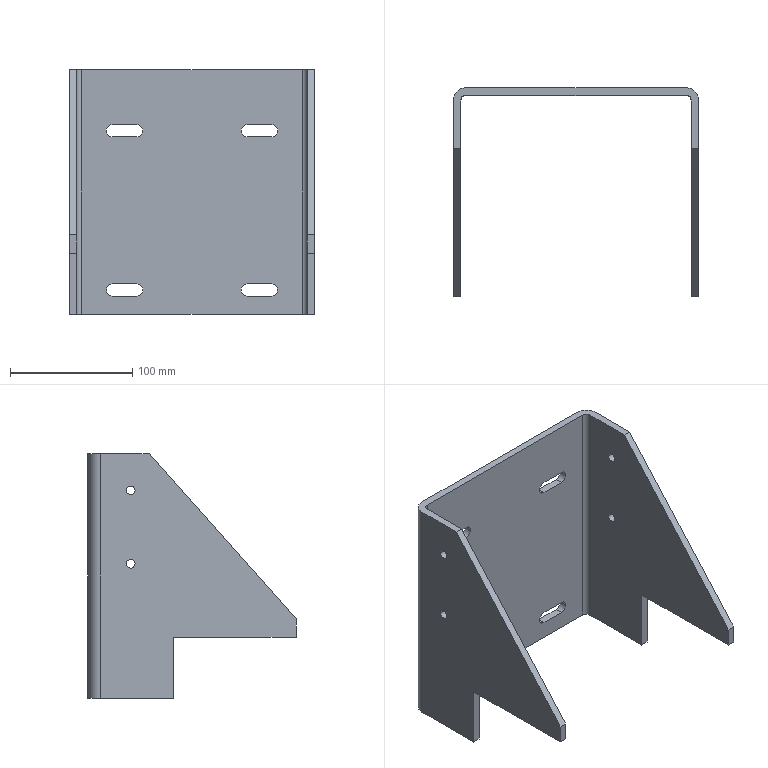Part | SolidWorks | features ICE 3, Extrusion 1 | 1 solid | 44 faces | box 200 x 170 x 200 mm | volume 461581 mm3 | plane 24 | cylinder 20 | commonest cylinder face diameters 7 x8 10 x8 8 x2 20 x2
STEP:
#1=CARTESIAN_POINT('',(0.,131.5,170.));
#2=VERTEX_POINT('',#1);
#3=CARTESIAN_POINT('',(0.,138.5,170.));
#4=VERTEX_POINT('',#3);
#5=CARTESIAN_POINT('',(0.,135.,170.));
#6=DIRECTION('',(1.,0.,0.));
#7=DIRECTION('',(0.,1.,0.));
#8=AXIS2_PLACEMENT_3D('',#5,#6,#7);
#9=CIRCLE('',#8,3.5);
#10=EDGE_CURVE('',#2,#4,#9,.T.);
#11=ORIENTED_EDGE('',*,*,#10,.F.);
#12=CARTESIAN_POINT('',(6.,131.5,170.));
#13=VERTEX_POINT('',#12);
#14=CARTESIAN_POINT('',(0.,131.5,170.));
#15=DIRECTION('',(1.,0.,0.));
#16=VECTOR('',#15,1000.);
#17=LINE('',#14,#16);
#18=EDGE_CURVE('',#2,#13,#17,.T.);
#19=ORIENTED_EDGE('',*,*,#18,.T.);
#20=CARTESIAN_POINT('',(6.,138.5,170.));
#21=VERTEX_POINT('',#20);
#22=CARTESIAN_POINT('',(6.,135.,170.));
#23=DIRECTION('',(-1.,0.,0.));
#24=DIRECTION('',(0.,0.,1.));
#25=AXIS2_PLACEMENT_3D('',#22,#23,#24);
#26=CIRCLE('',#25,3.5);
#27=EDGE_CURVE('',#21,#13,#26,.T.);
#28=ORIENTED_EDGE('',*,*,#27,.F.);
#29=CARTESIAN_POINT('',(0.,138.5,170.));
#30=DIRECTION('',(1.,0.,0.));
#31=VECTOR('',#30,1000.);
#32=LINE('',#29,#31);
#33=EDGE_CURVE('',#4,#21,#32,.T.);
#34=ORIENTED_EDGE('',*,*,#33,.F.);
#35=EDGE_LOOP('',(#11,#19,#28,#34));
#36=FACE_OUTER_BOUND('',#35,.T.);
#37=CARTESIAN_POINT('',(0.,135.,170.));
#38=DIRECTION('',(1.,0.,0.));
#39=DIRECTION('',(0.,1.,0.));
#40=AXIS2_PLACEMENT_3D('',#37,#38,#39);
#41=CYLINDRICAL_SURFACE('',#40,3.5);
#42=ADVANCED_FACE('',(#36),#41,.F.);
#43=CARTESIAN_POINT('',(0.,131.5,110.));
#44=VERTEX_POINT('',#43);
#45=CARTESIAN_POINT('',(0.,138.5,110.));
#46=VERTEX_POINT('',#45);
#47=CARTESIAN_POINT('',(0.,135.,110.));
#48=DIRECTION('',(1.,0.,0.));
#49=DIRECTION('',(0.,1.,0.));
#50=AXIS2_PLACEMENT_3D('',#47,#48,#49);
#51=CIRCLE('',#50,3.5);
#52=EDGE_CURVE('',#44,#46,#51,.T.);
#53=ORIENTED_EDGE('',*,*,#52,.F.);
#54=CARTESIAN_POINT('',(6.,131.5,110.));
#55=VERTEX_POINT('',#54);
#56=CARTESIAN_POINT('',(0.,131.5,110.));
#57=DIRECTION('',(1.,0.,0.));
#58=VECTOR('',#57,1000.);
#59=LINE('',#56,#58);
#60=EDGE_CURVE('',#44,#55,#59,.T.);
#61=ORIENTED_EDGE('',*,*,#60,.T.);
#62=CARTESIAN_POINT('',(6.,138.5,110.));
#63=VERTEX_POINT('',#62);
#64=CARTESIAN_POINT('',(6.,135.,110.));
#65=DIRECTION('',(-1.,0.,0.));
#66=DIRECTION('',(0.,0.,1.));
#67=AXIS2_PLACEMENT_3D('',#64,#65,#66);
#68=CIRCLE('',#67,3.5);
#69=EDGE_CURVE('',#63,#55,#68,.T.);
#70=ORIENTED_EDGE('',*,*,#69,.F.);
#71=CARTESIAN_POINT('',(0.,138.5,110.));
#72=DIRECTION('',(1.,0.,0.));
#73=VECTOR('',#72,1000.);
#74=LINE('',#71,#73);
#75=EDGE_CURVE('',#46,#63,#74,.T.);
#76=ORIENTED_EDGE('',*,*,#75,.F.);
#77=EDGE_LOOP('',(#53,#61,#70,#76));
#78=FACE_OUTER_BOUND('',#77,.T.);
#79=CARTESIAN_POINT('',(0.,135.,110.));
#80=DIRECTION('',(1.,0.,0.));
#81=DIRECTION('',(0.,1.,0.));
#82=AXIS2_PLACEMENT_3D('',#79,#80,#81);
#83=CYLINDRICAL_SURFACE('',#82,3.5);
#84=ADVANCED_FACE('',(#78),#83,.F.);
#85=CARTESIAN_POINT('',(194.,131.5,170.));
#86=VERTEX_POINT('',#85);
#87=CARTESIAN_POINT('',(194.,138.5,170.));
#88=VERTEX_POINT('',#87);
#89=CARTESIAN_POINT('',(194.,135.,170.));
#90=DIRECTION('',(1.,0.,0.));
#91=DIRECTION('',(0.,1.,0.));
#92=AXIS2_PLACEMENT_3D('',#89,#90,#91);
#93=CIRCLE('',#92,3.5);
#94=EDGE_CURVE('',#86,#88,#93,.T.);
#95=ORIENTED_EDGE('',*,*,#94,.F.);
#96=CARTESIAN_POINT('',(200.,131.5,170.));
#97=VERTEX_POINT('',#96);
#98=CARTESIAN_POINT('',(0.,131.5,170.));
#99=DIRECTION('',(1.,0.,0.));
#100=VECTOR('',#99,1000.);
#101=LINE('',#98,#100);
#102=EDGE_CURVE('',#86,#97,#101,.T.);
#103=ORIENTED_EDGE('',*,*,#102,.T.);
#104=CARTESIAN_POINT('',(200.,138.5,170.));
#105=VERTEX_POINT('',#104);
#106=CARTESIAN_POINT('',(200.,135.,170.));
#107=DIRECTION('',(1.,0.,0.));
#108=DIRECTION('',(0.,1.,0.));
#109=AXIS2_PLACEMENT_3D('',#106,#107,#108);
#110=CIRCLE('',#109,3.5);
#111=EDGE_CURVE('',#97,#105,#110,.T.);
#112=ORIENTED_EDGE('',*,*,#111,.T.);
#113=CARTESIAN_POINT('',(0.,138.5,170.));
#114=DIRECTION('',(1.,0.,0.));
#115=VECTOR('',#114,1000.);
#116=LINE('',#113,#115);
#117=EDGE_CURVE('',#88,#105,#116,.T.);
#118=ORIENTED_EDGE('',*,*,#117,.F.);
#119=EDGE_LOOP('',(#95,#103,#112,#118));
#120=FACE_OUTER_BOUND('',#119,.T.);
#121=CARTESIAN_POINT('',(0.,135.,170.));
#122=DIRECTION('',(1.,0.,0.));
#123=DIRECTION('',(0.,1.,0.));
#124=AXIS2_PLACEMENT_3D('',#121,#122,#123);
#125=CYLINDRICAL_SURFACE('',#124,3.5);
#126=ADVANCED_FACE('',(#120),#125,.F.);
#127=CARTESIAN_POINT('',(194.,131.5,110.));
#128=VERTEX_POINT('',#127);
#129=CARTESIAN_POINT('',(194.,138.5,110.));
#130=VERTEX_POINT('',#129);
#131=CARTESIAN_POINT('',(194.,135.,110.));
#132=DIRECTION('',(1.,0.,0.));
#133=DIRECTION('',(0.,1.,0.));
#134=AXIS2_PLACEMENT_3D('',#131,#132,#133);
#135=CIRCLE('',#134,3.5);
#136=EDGE_CURVE('',#128,#130,#135,.T.);
#137=ORIENTED_EDGE('',*,*,#136,.F.);
#138=CARTESIAN_POINT('',(200.,131.5,110.));
#139=VERTEX_POINT('',#138);
#140=CARTESIAN_POINT('',(0.,131.5,110.));
#141=DIRECTION('',(1.,0.,0.));
#142=VECTOR('',#141,1000.);
#143=LINE('',#140,#142);
#144=EDGE_CURVE('',#128,#139,#143,.T.);
#145=ORIENTED_EDGE('',*,*,#144,.T.);
#146=CARTESIAN_POINT('',(200.,138.5,110.));
#147=VERTEX_POINT('',#146);
#148=CARTESIAN_POINT('',(200.,135.,110.));
#149=DIRECTION('',(1.,0.,0.));
#150=DIRECTION('',(0.,1.,0.));
#151=AXIS2_PLACEMENT_3D('',#148,#149,#150);
#152=CIRCLE('',#151,3.5);
#153=EDGE_CURVE('',#139,#147,#152,.T.);
#154=ORIENTED_EDGE('',*,*,#153,.T.);
#155=CARTESIAN_POINT('',(0.,138.5,110.));
#156=DIRECTION('',(1.,0.,0.));
#157=VECTOR('',#156,1000.);
#158=LINE('',#155,#157);
#159=EDGE_CURVE('',#130,#147,#158,.T.);
#160=ORIENTED_EDGE('',*,*,#159,.F.);
#161=EDGE_LOOP('',(#137,#145,#154,#160));
#162=FACE_OUTER_BOUND('',#161,.T.);
#163=CARTESIAN_POINT('',(0.,135.,110.));
#164=DIRECTION('',(1.,0.,0.));
#165=DIRECTION('',(0.,1.,0.));
#166=AXIS2_PLACEMENT_3D('',#163,#164,#165);
#167=CYLINDRICAL_SURFACE('',#166,3.5);
#168=ADVANCED_FACE('',(#162),#167,.F.);
#169=CARTESIAN_POINT('',(200.,135.,170.));
#170=DIRECTION('',(1.,0.,0.));
#171=DIRECTION('',(0.,1.,0.));
#172=AXIS2_PLACEMENT_3D('',#169,#170,#171);
#173=CIRCLE('',#172,3.5);
#174=EDGE_CURVE('',#105,#97,#173,.T.);
#175=ORIENTED_EDGE('',*,*,#174,.F.);
#176=ORIENTED_EDGE('',*,*,#111,.F.);
#177=EDGE_LOOP('',(#175,#176));
#178=FACE_BOUND('',#177,.T.);
#179=CARTESIAN_POINT('',(200.,135.,110.));
#180=DIRECTION('',(1.,0.,0.));
#181=DIRECTION('',(0.,1.,0.));
#182=AXIS2_PLACEMENT_3D('',#179,#180,#181);
#183=CIRCLE('',#182,3.5);
#184=EDGE_CURVE('',#147,#139,#183,.T.);
#185=ORIENTED_EDGE('',*,*,#184,.F.);
#186=ORIENTED_EDGE('',*,*,#153,.F.);
#187=EDGE_LOOP('',(#185,#186));
#188=FACE_BOUND('',#187,.T.);
#189=CARTESIAN_POINT('',(200.,0.,65.));
#190=VERTEX_POINT('',#189);
#191=CARTESIAN_POINT('',(200.,120.,200.));
#192=VERTEX_POINT('',#191);
#193=CARTESIAN_POINT('',(200.,120.,200.));
#194=DIRECTION('',(0.,0.6644,0.7474));
#195=VECTOR('',#194,1000.);
#196=LINE('',#193,#195);
#197=EDGE_CURVE('',#190,#192,#196,.T.);
#198=ORIENTED_EDGE('',*,*,#197,.F.);
#199=CARTESIAN_POINT('',(200.,0.,50.));
#200=VERTEX_POINT('',#199);
#201=CARTESIAN_POINT('',(200.,0.,200.));
#202=DIRECTION('',(0.,0.,-1.));
#203=VECTOR('',#202,1000.);
#204=LINE('',#201,#203);
#205=EDGE_CURVE('',#190,#200,#204,.T.);
#206=ORIENTED_EDGE('',*,*,#205,.T.);
#207=CARTESIAN_POINT('',(200.,100.,50.));
#208=VERTEX_POINT('',#207);
#209=CARTESIAN_POINT('',(200.,0.,50.));
#210=DIRECTION('',(0.,-1.,0.));
#211=VECTOR('',#210,1000.);
#212=LINE('',#209,#211);
#213=EDGE_CURVE('',#208,#200,#212,.T.);
#214=ORIENTED_EDGE('',*,*,#213,.F.);
#215=CARTESIAN_POINT('',(200.,100.,0.));
#216=VERTEX_POINT('',#215);
#217=CARTESIAN_POINT('',(200.,100.,50.));
#218=DIRECTION('',(0.,0.,1.));
#219=VECTOR('',#218,1000.);
#220=LINE('',#217,#219);
#221=EDGE_CURVE('',#216,#208,#220,.T.);
#222=ORIENTED_EDGE('',*,*,#221,.F.);
#223=CARTESIAN_POINT('',(200.,160.,0.));
#224=VERTEX_POINT('',#223);
#225=CARTESIAN_POINT('',(200.,160.,0.));
#226=DIRECTION('',(0.,-1.,0.));
#227=VECTOR('',#226,1000.);
#228=LINE('',#225,#227);
#229=EDGE_CURVE('',#224,#216,#228,.T.);
#230=ORIENTED_EDGE('',*,*,#229,.F.);
#231=CARTESIAN_POINT('',(200.,160.,200.));
#232=VERTEX_POINT('',#231);
#233=CARTESIAN_POINT('',(200.,160.,200.));
#234=DIRECTION('',(0.,0.,-1.));
#235=VECTOR('',#234,1000.);
#236=LINE('',#233,#235);
#237=EDGE_CURVE('',#232,#224,#236,.T.);
#238=ORIENTED_EDGE('',*,*,#237,.F.);
#239=CARTESIAN_POINT('',(200.,160.,200.));
#240=DIRECTION('',(0.,-1.,0.));
#241=VECTOR('',#240,1000.);
#242=LINE('',#239,#241);
#243=EDGE_CURVE('',#232,#192,#242,.T.);
#244=ORIENTED_EDGE('',*,*,#243,.T.);
#245=EDGE_LOOP('',(#198,#206,#214,#222,#230,#238,#244));
#246=FACE_OUTER_BOUND('',#245,.T.);
#247=CARTESIAN_POINT('',(200.,160.,200.));
#248=DIRECTION('',(1.,0.,0.));
#249=DIRECTION('',(0.,0.,-1.));
#250=AXIS2_PLACEMENT_3D('',#247,#248,#249);
#251=PLANE('',#250);
#252=ADVANCED_FACE('',(#178,#188,#246),#251,.T.);
#253=CARTESIAN_POINT('',(190.,170.,0.));
#254=VERTEX_POINT('',#253);
#255=CARTESIAN_POINT('',(190.,160.,0.));
#256=DIRECTION('',(0.,0.,-1.));
#257=DIRECTION('',(-1.,0.,0.));
#258=AXIS2_PLACEMENT_3D('',#255,#256,#257);
#259=CIRCLE('',#258,10.);
#260=EDGE_CURVE('',#254,#224,#259,.T.);
#261=ORIENTED_EDGE('',*,*,#260,.F.);
#262=CARTESIAN_POINT('',(190.,170.,200.));
#263=VERTEX_POINT('',#262);
#264=CARTESIAN_POINT('',(190.,170.,200.));
#265=DIRECTION('',(0.,0.,-1.));
#266=VECTOR('',#265,1000.);
#267=LINE('',#264,#266);
#268=EDGE_CURVE('',#263,#254,#267,.T.);
#269=ORIENTED_EDGE('',*,*,#268,.F.);
#270=CARTESIAN_POINT('',(190.,160.,200.));
#271=DIRECTION('',(0.,0.,-1.));
#272=DIRECTION('',(-1.,0.,0.));
#273=AXIS2_PLACEMENT_3D('',#270,#271,#272);
#274=CIRCLE('',#273,10.);
#275=EDGE_CURVE('',#263,#232,#274,.T.);
#276=ORIENTED_EDGE('',*,*,#275,.T.);
#277=ORIENTED_EDGE('',*,*,#237,.T.);
#278=EDGE_LOOP('',(#261,#269,#276,#277));
#279=FACE_OUTER_BOUND('',#278,.T.);
#280=CARTESIAN_POINT('',(190.,160.,200.));
#281=DIRECTION('',(0.,0.,-1.));
#282=DIRECTION('',(-1.,0.,0.));
#283=AXIS2_PLACEMENT_3D('',#280,#281,#282);
#284=CYLINDRICAL_SURFACE('',#283,10.);
#285=ADVANCED_FACE('',(#279),#284,.T.);
#286=CARTESIAN_POINT('',(165.,170.,155.));
#287=VERTEX_POINT('',#286);
#288=CARTESIAN_POINT('',(165.,170.,145.));
#289=VERTEX_POINT('',#288);
#290=CARTESIAN_POINT('',(165.,170.,150.));
#291=DIRECTION('',(0.,1.,0.));
#292=DIRECTION('',(0.,0.,1.));
#293=AXIS2_PLACEMENT_3D('',#290,#291,#292);
#294=CIRCLE('',#293,5.);
#295=EDGE_CURVE('',#287,#289,#294,.T.);
#296=ORIENTED_EDGE('',*,*,#295,.F.);
#297=CARTESIAN_POINT('',(145.,170.,155.));
#298=VERTEX_POINT('',#297);
#299=CARTESIAN_POINT('',(165.,170.,155.));
#300=DIRECTION('',(1.,0.,0.));
#301=VECTOR('',#300,1000.);
#302=LINE('',#299,#301);
#303=EDGE_CURVE('',#298,#287,#302,.T.);
#304=ORIENTED_EDGE('',*,*,#303,.F.);
#305=CARTESIAN_POINT('',(145.,170.,145.));
#306=VERTEX_POINT('',#305);
#307=CARTESIAN_POINT('',(145.,170.,150.));
#308=DIRECTION('',(0.,1.,0.));
#309=DIRECTION('',(0.,0.,1.));
#310=AXIS2_PLACEMENT_3D('',#307,#308,#309);
#311=CIRCLE('',#310,5.);
#312=EDGE_CURVE('',#306,#298,#311,.T.);
#313=ORIENTED_EDGE('',*,*,#312,.F.);
#314=CARTESIAN_POINT('',(165.,170.,145.));
#315=DIRECTION('',(-1.,0.,0.));
#316=VECTOR('',#315,1000.);
#317=LINE('',#314,#316);
#318=EDGE_CURVE('',#289,#306,#317,.T.);
#319=ORIENTED_EDGE('',*,*,#318,.F.);
#320=EDGE_LOOP('',(#296,#304,#313,#319));
#321=FACE_BOUND('',#320,.T.);
#322=CARTESIAN_POINT('',(55.,170.,25.));
#323=VERTEX_POINT('',#322);
#324=CARTESIAN_POINT('',(55.,170.,15.));
#325=VERTEX_POINT('',#324);
#326=CARTESIAN_POINT('',(55.,170.,20.));
#327=DIRECTION('',(0.,1.,0.));
#328=DIRECTION('',(0.,0.,1.));
#329=AXIS2_PLACEMENT_3D('',#326,#327,#328);
#330=CIRCLE('',#329,5.);
#331=EDGE_CURVE('',#323,#325,#330,.T.);
#332=ORIENTED_EDGE('',*,*,#331,.F.);
#333=CARTESIAN_POINT('',(35.,170.,25.));
#334=VERTEX_POINT('',#333);
#335=CARTESIAN_POINT('',(55.,170.,25.));
#336=DIRECTION('',(1.,0.,0.));
#337=VECTOR('',#336,1000.);
#338=LINE('',#335,#337);
#339=EDGE_CURVE('',#334,#323,#338,.T.);
#340=ORIENTED_EDGE('',*,*,#339,.F.);
#341=CARTESIAN_POINT('',(35.,170.,15.));
#342=VERTEX_POINT('',#341);
#343=CARTESIAN_POINT('',(35.,170.,20.));
#344=DIRECTION('',(0.,1.,0.));
#345=DIRECTION('',(0.,0.,1.));
#346=AXIS2_PLACEMENT_3D('',#343,#344,#345);
#347=CIRCLE('',#346,5.);
#348=EDGE_CURVE('',#342,#334,#347,.T.);
#349=ORIENTED_EDGE('',*,*,#348,.F.);
#350=CARTESIAN_POINT('',(55.,170.,15.));
#351=DIRECTION('',(-1.,0.,0.));
#352=VECTOR('',#351,1000.);
#353=LINE('',#350,#352);
#354=EDGE_CURVE('',#325,#342,#353,.T.);
#355=ORIENTED_EDGE('',*,*,#354,.F.);
#356=EDGE_LOOP('',(#332,#340,#349,#355));
#357=FACE_BOUND('',#356,.T.);
#358=CARTESIAN_POINT('',(55.,170.,155.));
#359=VERTEX_POINT('',#358);
#360=CARTESIAN_POINT('',(55.,170.,145.));
#361=VERTEX_POINT('',#360);
#362=CARTESIAN_POINT('',(55.,170.,150.));
#363=DIRECTION('',(0.,1.,0.));
#364=DIRECTION('',(0.,0.,1.));
#365=AXIS2_PLACEMENT_3D('',#362,#363,#364);
#366=CIRCLE('',#365,5.);
#367=EDGE_CURVE('',#359,#361,#366,.T.);
#368=ORIENTED_EDGE('',*,*,#367,.F.);
#369=CARTESIAN_POINT('',(35.,170.,155.));
#370=VERTEX_POINT('',#369);
#371=CARTESIAN_POINT('',(55.,170.,155.));
#372=DIRECTION('',(1.,0.,0.));
#373=VECTOR('',#372,1000.);
#374=LINE('',#371,#373);
#375=EDGE_CURVE('',#370,#359,#374,.T.);
#376=ORIENTED_EDGE('',*,*,#375,.F.);
#377=CARTESIAN_POINT('',(35.,170.,145.));
#378=VERTEX_POINT('',#377);
#379=CARTESIAN_POINT('',(35.,170.,150.));
#380=DIRECTION('',(0.,1.,0.));
#381=DIRECTION('',(0.,0.,1.));
#382=AXIS2_PLACEMENT_3D('',#379,#380,#381);
#383=CIRCLE('',#382,5.);
#384=EDGE_CURVE('',#378,#370,#383,.T.);
#385=ORIENTED_EDGE('',*,*,#384,.F.);
#386=CARTESIAN_POINT('',(55.,170.,145.));
#387=DIRECTION('',(-1.,0.,0.));
#388=VECTOR('',#387,1000.);
#389=LINE('',#386,#388);
#390=EDGE_CURVE('',#361,#378,#389,.T.);
#391=ORIENTED_EDGE('',*,*,#390,.F.);
#392=EDGE_LOOP('',(#368,#376,#385,#391));
#393=FACE_BOUND('',#392,.T.);
#394=CARTESIAN_POINT('',(165.,170.,25.));
#395=VERTEX_POINT('',#394);
#396=CARTESIAN_POINT('',(165.,170.,15.));
#397=VERTEX_POINT('',#396);
#398=CARTESIAN_POINT('',(165.,170.,20.));
#399=DIRECTION('',(0.,1.,0.));
#400=DIRECTION('',(0.,0.,1.));
#401=AXIS2_PLACEMENT_3D('',#398,#399,#400);
#402=CIRCLE('',#401,5.);
#403=EDGE_CURVE('',#395,#397,#402,.T.);
#404=ORIENTED_EDGE('',*,*,#403,.F.);
#405=CARTESIAN_POINT('',(145.,170.,25.));
#406=VERTEX_POINT('',#405);
#407=CARTESIAN_POINT('',(165.,170.,25.));
#408=DIRECTION('',(1.,0.,0.));
#409=VECTOR('',#408,1000.);
#410=LINE('',#407,#409);
#411=EDGE_CURVE('',#406,#395,#410,.T.);
#412=ORIENTED_EDGE('',*,*,#411,.F.);
#413=CARTESIAN_POINT('',(145.,170.,15.));
#414=VERTEX_POINT('',#413);
#415=CARTESIAN_POINT('',(145.,170.,20.));
#416=DIRECTION('',(0.,1.,0.));
#417=DIRECTION('',(0.,0.,1.));
#418=AXIS2_PLACEMENT_3D('',#415,#416,#417);
#419=CIRCLE('',#418,5.);
#420=EDGE_CURVE('',#414,#406,#419,.T.);
#421=ORIENTED_EDGE('',*,*,#420,.F.);
#422=CARTESIAN_POINT('',(165.,170.,15.));
#423=DIRECTION('',(-1.,0.,0.));
#424=VECTOR('',#423,1000.);
#425=LINE('',#422,#424);
#426=EDGE_CURVE('',#397,#414,#425,.T.);
#427=ORIENTED_EDGE('',*,*,#426,.F.);
#428=EDGE_LOOP('',(#404,#412,#421,#427));
#429=FACE_BOUND('',#428,.T.);
#430=CARTESIAN_POINT('',(10.,170.,0.));
#431=VERTEX_POINT('',#430);
#432=CARTESIAN_POINT('',(10.,170.,0.));
#433=DIRECTION('',(1.,0.,0.));
#434=VECTOR('',#433,1000.);
#435=LINE('',#432,#434);
#436=EDGE_CURVE('',#431,#254,#435,.T.);
#437=ORIENTED_EDGE('',*,*,#436,.F.);
#438=CARTESIAN_POINT('',(10.,170.,200.));
#439=VERTEX_POINT('',#438);
#440=CARTESIAN_POINT('',(10.,170.,200.));
#441=DIRECTION('',(0.,0.,-1.));
#442=VECTOR('',#441,1000.);
#443=LINE('',#440,#442);
#444=EDGE_CURVE('',#439,#431,#443,.T.);
#445=ORIENTED_EDGE('',*,*,#444,.F.);
#446=CARTESIAN_POINT('',(10.,170.,200.));
#447=DIRECTION('',(1.,0.,0.));
#448=VECTOR('',#447,1000.);
#449=LINE('',#446,#448);
#450=EDGE_CURVE('',#439,#263,#449,.T.);
#451=ORIENTED_EDGE('',*,*,#450,.T.);
#452=ORIENTED_EDGE('',*,*,#268,.T.);
#453=EDGE_LOOP('',(#437,#445,#451,#452));
#454=FACE_OUTER_BOUND('',#453,.T.);
#455=CARTESIAN_POINT('',(10.,170.,200.));
#456=DIRECTION('',(0.,1.,0.));
#457=DIRECTION('',(0.,0.,1.));
#458=AXIS2_PLACEMENT_3D('',#455,#456,#457);
#459=PLANE('',#458);
#460=ADVANCED_FACE('',(#321,#357,#393,#429,#454),#459,.T.);
#461=CARTESIAN_POINT('',(0.,160.,0.));
#462=VERTEX_POINT('',#461);
#463=CARTESIAN_POINT('',(10.,160.,0.));
#464=DIRECTION('',(0.,0.,-1.));
#465=DIRECTION('',(-1.,0.,0.));
#466=AXIS2_PLACEMENT_3D('',#463,#464,#465);
#467=CIRCLE('',#466,10.);
#468=EDGE_CURVE('',#462,#431,#467,.T.);
#469=ORIENTED_EDGE('',*,*,#468,.F.);
#470=CARTESIAN_POINT('',(0.,160.,200.));
#471=VERTEX_POINT('',#470);
#472=CARTESIAN_POINT('',(0.,160.,200.));
#473=DIRECTION('',(0.,0.,-1.));
#474=VECTOR('',#473,1000.);
#475=LINE('',#472,#474);
#476=EDGE_CURVE('',#471,#462,#475,.T.);
#477=ORIENTED_EDGE('',*,*,#476,.F.);
#478=CARTESIAN_POINT('',(10.,160.,200.));
#479=DIRECTION('',(0.,0.,-1.));
#480=DIRECTION('',(-1.,0.,0.));
#481=AXIS2_PLACEMENT_3D('',#478,#479,#480);
#482=CIRCLE('',#481,10.);
#483=EDGE_CURVE('',#471,#439,#482,.T.);
#484=ORIENTED_EDGE('',*,*,#483,.T.);
#485=ORIENTED_EDGE('',*,*,#444,.T.);
#486=EDGE_LOOP('',(#469,#477,#484,#485));
#487=FACE_OUTER_BOUND('',#486,.T.);
#488=CARTESIAN_POINT('',(10.,160.,200.));
#489=DIRECTION('',(0.,0.,-1.));
#490=DIRECTION('',(-1.,0.,0.));
#491=AXIS2_PLACEMENT_3D('',#488,#489,#490);
#492=CYLINDRICAL_SURFACE('',#491,10.);
#493=ADVANCED_FACE('',(#487),#492,.T.);
#494=CARTESIAN_POINT('',(0.,135.,170.));
#495=DIRECTION('',(1.,0.,0.));
#496=DIRECTION('',(0.,1.,0.));
#497=AXIS2_PLACEMENT_3D('',#494,#495,#496);
#498=CIRCLE('',#497,3.5);
#499=EDGE_CURVE('',#4,#2,#498,.T.);
#500=ORIENTED_EDGE('',*,*,#499,.T.);
#501=ORIENTED_EDGE('',*,*,#10,.T.);
#502=EDGE_LOOP('',(#500,#501));
#503=FACE_BOUND('',#502,.T.);
#504=CARTESIAN_POINT('',(0.,135.,110.));
#505=DIRECTION('',(1.,0.,0.));
#506=DIRECTION('',(0.,1.,0.));
#507=AXIS2_PLACEMENT_3D('',#504,#505,#506);
#508=CIRCLE('',#507,3.5);
#509=EDGE_CURVE('',#46,#44,#508,.T.);
#510=ORIENTED_EDGE('',*,*,#509,.T.);
#511=ORIENTED_EDGE('',*,*,#52,.T.);
#512=EDGE_LOOP('',(#510,#511));
#513=FACE_BOUND('',#512,.T.);
#514=CARTESIAN_POINT('',(0.,0.,65.));
#515=VERTEX_POINT('',#514);
#516=CARTESIAN_POINT('',(0.,120.,200.));
#517=VERTEX_POINT('',#516);
#518=CARTESIAN_POINT('',(0.,120.,200.));
#519=DIRECTION('',(0.,0.6644,0.7474));
#520=VECTOR('',#519,1000.);
#521=LINE('',#518,#520);
#522=EDGE_CURVE('',#515,#517,#521,.T.);
#523=ORIENTED_EDGE('',*,*,#522,.T.);
#524=CARTESIAN_POINT('',(0.,0.,200.));
#525=DIRECTION('',(0.,1.,0.));
#526=VECTOR('',#525,1000.);
#527=LINE('',#524,#526);
#528=EDGE_CURVE('',#517,#471,#527,.T.);
#529=ORIENTED_EDGE('',*,*,#528,.T.);
#530=ORIENTED_EDGE('',*,*,#476,.T.);
#531=CARTESIAN_POINT('',(0.,100.,0.));
#532=VERTEX_POINT('',#531);
#533=CARTESIAN_POINT('',(0.,0.,0.));
#534=DIRECTION('',(0.,1.,0.));
#535=VECTOR('',#534,1000.);
#536=LINE('',#533,#535);
#537=EDGE_CURVE('',#532,#462,#536,.T.);
#538=ORIENTED_EDGE('',*,*,#537,.F.);
#539=CARTESIAN_POINT('',(0.,100.,50.));
#540=VERTEX_POINT('',#539);
#541=CARTESIAN_POINT('',(0.,100.,50.));
#542=DIRECTION('',(0.,0.,1.));
#543=VECTOR('',#542,1000.);
#544=LINE('',#541,#543);
#545=EDGE_CURVE('',#532,#540,#544,.T.);
#546=ORIENTED_EDGE('',*,*,#545,.T.);
#547=CARTESIAN_POINT('',(0.,0.,50.));
#548=VERTEX_POINT('',#547);
#549=CARTESIAN_POINT('',(0.,0.,50.));
#550=DIRECTION('',(0.,-1.,0.));
#551=VECTOR('',#550,1000.);
#552=LINE('',#549,#551);
#553=EDGE_CURVE('',#540,#548,#552,.T.);
#554=ORIENTED_EDGE('',*,*,#553,.T.);
#555=CARTESIAN_POINT('',(0.,0.,200.));
#556=DIRECTION('',(0.,0.,-1.));
#557=VECTOR('',#556,1000.);
#558=LINE('',#555,#557);
#559=EDGE_CURVE('',#515,#548,#558,.T.);
#560=ORIENTED_EDGE('',*,*,#559,.F.);
#561=EDGE_LOOP('',(#523,#529,#530,#538,#546,#554,#560));
#562=FACE_OUTER_BOUND('',#561,.T.);
#563=CARTESIAN_POINT('',(0.,0.,200.));
#564=DIRECTION('',(-1.,0.,0.));
#565=DIRECTION('',(0.,0.,1.));
#566=AXIS2_PLACEMENT_3D('',#563,#564,#565);
#567=PLANE('',#566);
#568=ADVANCED_FACE('',(#503,#513,#562),#567,.T.);
#569=CARTESIAN_POINT('',(6.,0.,65.));
#570=VERTEX_POINT('',#569);
#571=CARTESIAN_POINT('',(0.,0.,65.));
#572=DIRECTION('',(1.,0.,0.));
#573=VECTOR('',#572,1000.);
#574=LINE('',#571,#573);
#575=EDGE_CURVE('',#515,#570,#574,.T.);
#576=ORIENTED_EDGE('',*,*,#575,.F.);
#577=ORIENTED_EDGE('',*,*,#559,.T.);
#578=CARTESIAN_POINT('',(6.,0.,50.));
#579=VERTEX_POINT('',#578);
#580=CARTESIAN_POINT('',(0.,0.,50.));
#581=DIRECTION('',(1.,0.,0.));
#582=VECTOR('',#581,1000.);
#583=LINE('',#580,#582);
#584=EDGE_CURVE('',#548,#579,#583,.T.);
#585=ORIENTED_EDGE('',*,*,#584,.T.);
#586=CARTESIAN_POINT('',(6.,0.,200.));
#587=DIRECTION('',(0.,0.,-1.));
#588=VECTOR('',#587,1000.);
#589=LINE('',#586,#588);
#590=EDGE_CURVE('',#570,#579,#589,.T.);
#591=ORIENTED_EDGE('',*,*,#590,.F.);
#592=EDGE_LOOP('',(#576,#577,#585,#591));
#593=FACE_OUTER_BOUND('',#592,.T.);
#594=CARTESIAN_POINT('',(6.,0.,200.));
#595=DIRECTION('',(0.,-1.,0.));
#596=DIRECTION('',(0.,0.,-1.));
#597=AXIS2_PLACEMENT_3D('',#594,#595,#596);
#598=PLANE('',#597);
#599=ADVANCED_FACE('',(#593),#598,.T.);
#600=ORIENTED_EDGE('',*,*,#27,.T.);
#601=CARTESIAN_POINT('',(6.,135.,170.));
#602=DIRECTION('',(-1.,0.,0.));
#603=DIRECTION('',(0.,0.,1.));
#604=AXIS2_PLACEMENT_3D('',#601,#602,#603);
#605=CIRCLE('',#604,3.5);
#606=EDGE_CURVE('',#13,#21,#605,.T.);
#607=ORIENTED_EDGE('',*,*,#606,.T.);
#608=EDGE_LOOP('',(#600,#607));
#609=FACE_BOUND('',#608,.T.);
#610=ORIENTED_EDGE('',*,*,#69,.T.);
#611=CARTESIAN_POINT('',(6.,135.,110.));
#612=DIRECTION('',(-1.,0.,0.));
#613=DIRECTION('',(0.,0.,1.));
#614=AXIS2_PLACEMENT_3D('',#611,#612,#613);
#615=CIRCLE('',#614,3.5);
#616=EDGE_CURVE('',#55,#63,#615,.T.);
#617=ORIENTED_EDGE('',*,*,#616,.T.);
#618=EDGE_LOOP('',(#610,#617));
#619=FACE_BOUND('',#618,.T.);
#620=CARTESIAN_POINT('',(6.,120.,200.));
#621=VERTEX_POINT('',#620);
#622=CARTESIAN_POINT('',(6.,160.,200.));
#623=VERTEX_POINT('',#622);
#624=CARTESIAN_POINT('',(6.,0.,200.));
#625=DIRECTION('',(0.,1.,0.));
#626=VECTOR('',#625,1000.);
#627=LINE('',#624,#626);
#628=EDGE_CURVE('',#621,#623,#627,.T.);
#629=ORIENTED_EDGE('',*,*,#628,.F.);
#630=CARTESIAN_POINT('',(6.,67.034,140.414));
#631=DIRECTION('',(0.,-0.6644,-0.7474));
#632=VECTOR('',#631,1000.);
#633=LINE('',#630,#632);
#634=EDGE_CURVE('',#621,#570,#633,.T.);
#635=ORIENTED_EDGE('',*,*,#634,.T.);
#636=ORIENTED_EDGE('',*,*,#590,.T.);
#637=CARTESIAN_POINT('',(6.,100.,50.));
#638=VERTEX_POINT('',#637);
#639=CARTESIAN_POINT('',(6.,0.,50.));
#640=DIRECTION('',(0.,1.,0.));
#641=VECTOR('',#640,1000.);
#642=LINE('',#639,#641);
#643=EDGE_CURVE('',#579,#638,#642,.T.);
#644=ORIENTED_EDGE('',*,*,#643,.T.);
#645=CARTESIAN_POINT('',(6.,100.,0.));
#646=VERTEX_POINT('',#645);
#647=CARTESIAN_POINT('',(6.,100.,200.));
#648=DIRECTION('',(0.,0.,-1.));
#649=VECTOR('',#648,1000.);
#650=LINE('',#647,#649);
#651=EDGE_CURVE('',#638,#646,#650,.T.);
#652=ORIENTED_EDGE('',*,*,#651,.T.);
#653=CARTESIAN_POINT('',(6.,160.,0.));
#654=VERTEX_POINT('',#653);
#655=CARTESIAN_POINT('',(6.,0.,0.));
#656=DIRECTION('',(0.,1.,0.));
#657=VECTOR('',#656,1000.);
#658=LINE('',#655,#657);
#659=EDGE_CURVE('',#646,#654,#658,.T.);
#660=ORIENTED_EDGE('',*,*,#659,.T.);
#661=CARTESIAN_POINT('',(6.,160.,200.));
#662=DIRECTION('',(0.,0.,-1.));
#663=VECTOR('',#662,1000.);
#664=LINE('',#661,#663);
#665=EDGE_CURVE('',#623,#654,#664,.T.);
#666=ORIENTED_EDGE('',*,*,#665,.F.);
#667=EDGE_LOOP('',(#629,#635,#636,#644,#652,#660,#666));
#668=FACE_OUTER_BOUND('',#667,.T.);
#669=CARTESIAN_POINT('',(6.,0.,200.));
#670=DIRECTION('',(-1.,0.,0.));
#671=DIRECTION('',(0.,0.,1.));
#672=AXIS2_PLACEMENT_3D('',#669,#670,#671);
#673=PLANE('',#672);
#674=ADVANCED_FACE('',(#609,#619,#668),#673,.F.);
#675=CARTESIAN_POINT('',(10.,164.,0.));
#676=VERTEX_POINT('',#675);
#677=CARTESIAN_POINT('',(10.,160.,0.));
#678=DIRECTION('',(0.,0.,-1.));
#679=DIRECTION('',(-1.,0.,0.));
#680=AXIS2_PLACEMENT_3D('',#677,#678,#679);
#681=CIRCLE('',#680,4.);
#682=EDGE_CURVE('',#654,#676,#681,.T.);
#683=ORIENTED_EDGE('',*,*,#682,.T.);
#684=CARTESIAN_POINT('',(10.,164.,200.));
#685=VERTEX_POINT('',#684);
#686=CARTESIAN_POINT('',(10.,164.,200.));
#687=DIRECTION('',(0.,0.,-1.));
#688=VECTOR('',#687,1000.);
#689=LINE('',#686,#688);
#690=EDGE_CURVE('',#685,#676,#689,.T.);
#691=ORIENTED_EDGE('',*,*,#690,.F.);
#692=CARTESIAN_POINT('',(10.,160.,200.));
#693=DIRECTION('',(0.,0.,-1.));
#694=DIRECTION('',(-1.,0.,0.));
#695=AXIS2_PLACEMENT_3D('',#692,#693,#694);
#696=CIRCLE('',#695,4.);
#697=EDGE_CURVE('',#623,#685,#696,.T.);
#698=ORIENTED_EDGE('',*,*,#697,.F.);
#699=ORIENTED_EDGE('',*,*,#665,.T.);
#700=EDGE_LOOP('',(#683,#691,#698,#699));
#701=FACE_OUTER_BOUND('',#700,.T.);
#702=CARTESIAN_POINT('',(10.,160.,200.));
#703=DIRECTION('',(0.,0.,-1.));
#704=DIRECTION('',(-1.,0.,0.));
#705=AXIS2_PLACEMENT_3D('',#702,#703,#704);
#706=CYLINDRICAL_SURFACE('',#705,4.);
#707=ADVANCED_FACE('',(#701),#706,.F.);
#708=CARTESIAN_POINT('',(145.,164.,155.));
#709=VERTEX_POINT('',#708);
#710=CARTESIAN_POINT('',(165.,164.,155.));
#711=VERTEX_POINT('',#710);
#712=CARTESIAN_POINT('',(10.,164.,155.));
#713=DIRECTION('',(1.,0.,0.));
#714=VECTOR('',#713,1000.);
#715=LINE('',#712,#714);
#716=EDGE_CURVE('',#709,#711,#715,.T.);
#717=ORIENTED_EDGE('',*,*,#716,.T.);
#718=CARTESIAN_POINT('',(165.,164.,145.));
#719=VERTEX_POINT('',#718);
#720=CARTESIAN_POINT('',(165.,164.,150.));
#721=DIRECTION('',(0.,1.,0.));
#722=DIRECTION('',(0.,0.,1.));
#723=AXIS2_PLACEMENT_3D('',#720,#721,#722);
#724=CIRCLE('',#723,5.);
#725=EDGE_CURVE('',#711,#719,#724,.T.);
#726=ORIENTED_EDGE('',*,*,#725,.T.);
#727=CARTESIAN_POINT('',(145.,164.,145.));
#728=VERTEX_POINT('',#727);
#729=CARTESIAN_POINT('',(10.,164.,145.));
#730=DIRECTION('',(-1.,0.,0.));
#731=VECTOR('',#730,1000.);
#732=LINE('',#729,#731);
#733=EDGE_CURVE('',#719,#728,#732,.T.);
#734=ORIENTED_EDGE('',*,*,#733,.T.);
#735=CARTESIAN_POINT('',(145.,164.,150.));
#736=DIRECTION('',(0.,1.,0.));
#737=DIRECTION('',(0.,0.,1.));
#738=AXIS2_PLACEMENT_3D('',#735,#736,#737);
#739=CIRCLE('',#738,5.);
#740=EDGE_CURVE('',#728,#709,#739,.T.);
#741=ORIENTED_EDGE('',*,*,#740,.T.);
#742=EDGE_LOOP('',(#717,#726,#734,#741));
#743=FACE_BOUND('',#742,.T.);
#744=CARTESIAN_POINT('',(35.,164.,25.));
#745=VERTEX_POINT('',#744);
#746=CARTESIAN_POINT('',(55.,164.,25.));
#747=VERTEX_POINT('',#746);
#748=CARTESIAN_POINT('',(10.,164.,25.));
#749=DIRECTION('',(1.,0.,0.));
#750=VECTOR('',#749,1000.);
#751=LINE('',#748,#750);
#752=EDGE_CURVE('',#745,#747,#751,.T.);
#753=ORIENTED_EDGE('',*,*,#752,.T.);
#754=CARTESIAN_POINT('',(55.,164.,15.));
#755=VERTEX_POINT('',#754);
#756=CARTESIAN_POINT('',(55.,164.,20.));
#757=DIRECTION('',(0.,1.,0.));
#758=DIRECTION('',(0.,0.,1.));
#759=AXIS2_PLACEMENT_3D('',#756,#757,#758);
#760=CIRCLE('',#759,5.);
#761=EDGE_CURVE('',#747,#755,#760,.T.);
#762=ORIENTED_EDGE('',*,*,#761,.T.);
#763=CARTESIAN_POINT('',(35.,164.,15.));
#764=VERTEX_POINT('',#763);
#765=CARTESIAN_POINT('',(10.,164.,15.));
#766=DIRECTION('',(-1.,0.,0.));
#767=VECTOR('',#766,1000.);
#768=LINE('',#765,#767);
#769=EDGE_CURVE('',#755,#764,#768,.T.);
#770=ORIENTED_EDGE('',*,*,#769,.T.);
#771=CARTESIAN_POINT('',(35.,164.,20.));
#772=DIRECTION('',(0.,1.,0.));
#773=DIRECTION('',(0.,0.,1.));
#774=AXIS2_PLACEMENT_3D('',#771,#772,#773);
#775=CIRCLE('',#774,5.);
#776=EDGE_CURVE('',#764,#745,#775,.T.);
#777=ORIENTED_EDGE('',*,*,#776,.T.);
#778=EDGE_LOOP('',(#753,#762,#770,#777));
#779=FACE_BOUND('',#778,.T.);
#780=CARTESIAN_POINT('',(35.,164.,155.));
#781=VERTEX_POINT('',#780);
#782=CARTESIAN_POINT('',(55.,164.,155.));
#783=VERTEX_POINT('',#782);
#784=CARTESIAN_POINT('',(10.,164.,155.));
#785=DIRECTION('',(1.,0.,0.));
#786=VECTOR('',#785,1000.);
#787=LINE('',#784,#786);
#788=EDGE_CURVE('',#781,#783,#787,.T.);
#789=ORIENTED_EDGE('',*,*,#788,.T.);
#790=CARTESIAN_POINT('',(55.,164.,145.));
#791=VERTEX_POINT('',#790);
#792=CARTESIAN_POINT('',(55.,164.,150.));
#793=DIRECTION('',(0.,1.,0.));
#794=DIRECTION('',(0.,0.,1.));
#795=AXIS2_PLACEMENT_3D('',#792,#793,#794);
#796=CIRCLE('',#795,5.);
#797=EDGE_CURVE('',#783,#791,#796,.T.);
#798=ORIENTED_EDGE('',*,*,#797,.T.);
#799=CARTESIAN_POINT('',(35.,164.,145.));
#800=VERTEX_POINT('',#799);
#801=CARTESIAN_POINT('',(10.,164.,145.));
#802=DIRECTION('',(-1.,0.,0.));
#803=VECTOR('',#802,1000.);
#804=LINE('',#801,#803);
#805=EDGE_CURVE('',#791,#800,#804,.T.);
#806=ORIENTED_EDGE('',*,*,#805,.T.);
#807=CARTESIAN_POINT('',(35.,164.,150.));
#808=DIRECTION('',(0.,1.,0.));
#809=DIRECTION('',(0.,0.,1.));
#810=AXIS2_PLACEMENT_3D('',#807,#808,#809);
#811=CIRCLE('',#810,5.);
#812=EDGE_CURVE('',#800,#781,#811,.T.);
#813=ORIENTED_EDGE('',*,*,#812,.T.);
#814=EDGE_LOOP('',(#789,#798,#806,#813));
#815=FACE_BOUND('',#814,.T.);
#816=CARTESIAN_POINT('',(145.,164.,25.));
#817=VERTEX_POINT('',#816);
#818=CARTESIAN_POINT('',(165.,164.,25.));
#819=VERTEX_POINT('',#818);
#820=CARTESIAN_POINT('',(10.,164.,25.));
#821=DIRECTION('',(1.,0.,0.));
#822=VECTOR('',#821,1000.);
#823=LINE('',#820,#822);
#824=EDGE_CURVE('',#817,#819,#823,.T.);
#825=ORIENTED_EDGE('',*,*,#824,.T.);
#826=CARTESIAN_POINT('',(165.,164.,15.));
#827=VERTEX_POINT('',#826);
#828=CARTESIAN_POINT('',(165.,164.,20.));
#829=DIRECTION('',(0.,1.,0.));
#830=DIRECTION('',(0.,0.,1.));
#831=AXIS2_PLACEMENT_3D('',#828,#829,#830);
#832=CIRCLE('',#831,5.);
#833=EDGE_CURVE('',#819,#827,#832,.T.);
#834=ORIENTED_EDGE('',*,*,#833,.T.);
#835=CARTESIAN_POINT('',(145.,164.,15.));
#836=VERTEX_POINT('',#835);
#837=CARTESIAN_POINT('',(10.,164.,15.));
#838=DIRECTION('',(-1.,0.,0.));
#839=VECTOR('',#838,1000.);
#840=LINE('',#837,#839);
#841=EDGE_CURVE('',#827,#836,#840,.T.);
#842=ORIENTED_EDGE('',*,*,#841,.T.);
#843=CARTESIAN_POINT('',(145.,164.,20.));
#844=DIRECTION('',(0.,1.,0.));
#845=DIRECTION('',(0.,0.,1.));
#846=AXIS2_PLACEMENT_3D('',#843,#844,#845);
#847=CIRCLE('',#846,5.);
#848=EDGE_CURVE('',#836,#817,#847,.T.);
#849=ORIENTED_EDGE('',*,*,#848,.T.);
#850=EDGE_LOOP('',(#825,#834,#842,#849));
#851=FACE_BOUND('',#850,.T.);
#852=CARTESIAN_POINT('',(190.,164.,0.));
#853=VERTEX_POINT('',#852);
#854=CARTESIAN_POINT('',(10.,164.,0.));
#855=DIRECTION('',(1.,0.,0.));
#856=VECTOR('',#855,1000.);
#857=LINE('',#854,#856);
#858=EDGE_CURVE('',#676,#853,#857,.T.);
#859=ORIENTED_EDGE('',*,*,#858,.T.);
#860=CARTESIAN_POINT('',(190.,164.,200.));
#861=VERTEX_POINT('',#860);
#862=CARTESIAN_POINT('',(190.,164.,200.));
#863=DIRECTION('',(0.,0.,-1.));
#864=VECTOR('',#863,1000.);
#865=LINE('',#862,#864);
#866=EDGE_CURVE('',#861,#853,#865,.T.);
#867=ORIENTED_EDGE('',*,*,#866,.F.);
#868=CARTESIAN_POINT('',(10.,164.,200.));
#869=DIRECTION('',(1.,0.,0.));
#870=VECTOR('',#869,1000.);
#871=LINE('',#868,#870);
#872=EDGE_CURVE('',#685,#861,#871,.T.);
#873=ORIENTED_EDGE('',*,*,#872,.F.);
#874=ORIENTED_EDGE('',*,*,#690,.T.);
#875=EDGE_LOOP('',(#859,#867,#873,#874));
#876=FACE_OUTER_BOUND('',#875,.T.);
#877=CARTESIAN_POINT('',(10.,164.,200.));
#878=DIRECTION('',(0.,1.,0.));
#879=DIRECTION('',(0.,0.,1.));
#880=AXIS2_PLACEMENT_3D('',#877,#878,#879);
#881=PLANE('',#880);
#882=ADVANCED_FACE('',(#743,#779,#815,#851,#876),#881,.F.);
#883=CARTESIAN_POINT('',(194.,160.,0.));
#884=VERTEX_POINT('',#883);
#885=CARTESIAN_POINT('',(190.,160.,0.));
#886=DIRECTION('',(0.,0.,-1.));
#887=DIRECTION('',(-1.,0.,0.));
#888=AXIS2_PLACEMENT_3D('',#885,#886,#887);
#889=CIRCLE('',#888,4.);
#890=EDGE_CURVE('',#853,#884,#889,.T.);
#891=ORIENTED_EDGE('',*,*,#890,.T.);
#892=CARTESIAN_POINT('',(194.,160.,200.));
#893=VERTEX_POINT('',#892);
#894=CARTESIAN_POINT('',(194.,160.,200.));
#895=DIRECTION('',(0.,0.,-1.));
#896=VECTOR('',#895,1000.);
#897=LINE('',#894,#896);
#898=EDGE_CURVE('',#893,#884,#897,.T.);
#899=ORIENTED_EDGE('',*,*,#898,.F.);
#900=CARTESIAN_POINT('',(190.,160.,200.));
#901=DIRECTION('',(0.,0.,-1.));
#902=DIRECTION('',(-1.,0.,0.));
#903=AXIS2_PLACEMENT_3D('',#900,#901,#902);
#904=CIRCLE('',#903,4.);
#905=EDGE_CURVE('',#861,#893,#904,.T.);
#906=ORIENTED_EDGE('',*,*,#905,.F.);
#907=ORIENTED_EDGE('',*,*,#866,.T.);
#908=EDGE_LOOP('',(#891,#899,#906,#907));
#909=FACE_OUTER_BOUND('',#908,.T.);
#910=CARTESIAN_POINT('',(190.,160.,200.));
#911=DIRECTION('',(0.,0.,-1.));
#912=DIRECTION('',(-1.,0.,0.));
#913=AXIS2_PLACEMENT_3D('',#910,#911,#912);
#914=CYLINDRICAL_SURFACE('',#913,4.);
#915=ADVANCED_FACE('',(#909),#914,.F.);
#916=CARTESIAN_POINT('',(194.,135.,170.));
#917=DIRECTION('',(1.,0.,0.));
#918=DIRECTION('',(0.,1.,0.));
#919=AXIS2_PLACEMENT_3D('',#916,#917,#918);
#920=CIRCLE('',#919,3.5);
#921=EDGE_CURVE('',#88,#86,#920,.T.);
#922=ORIENTED_EDGE('',*,*,#921,.T.);
#923=ORIENTED_EDGE('',*,*,#94,.T.);
#924=EDGE_LOOP('',(#922,#923));
#925=FACE_BOUND('',#924,.T.);
#926=CARTESIAN_POINT('',(194.,135.,110.));
#927=DIRECTION('',(1.,0.,0.));
#928=DIRECTION('',(0.,1.,0.));
#929=AXIS2_PLACEMENT_3D('',#926,#927,#928);
#930=CIRCLE('',#929,3.5);
#931=EDGE_CURVE('',#130,#128,#930,.T.);
#932=ORIENTED_EDGE('',*,*,#931,.T.);
#933=ORIENTED_EDGE('',*,*,#136,.T.);
#934=EDGE_LOOP('',(#932,#933));
#935=FACE_BOUND('',#934,.T.);
#936=CARTESIAN_POINT('',(194.,0.,65.));
#937=VERTEX_POINT('',#936);
#938=CARTESIAN_POINT('',(194.,0.,50.));
#939=VERTEX_POINT('',#938);
#940=CARTESIAN_POINT('',(194.,0.,200.));
#941=DIRECTION('',(0.,0.,-1.));
#942=VECTOR('',#941,1000.);
#943=LINE('',#940,#942);
#944=EDGE_CURVE('',#937,#939,#943,.T.);
#945=ORIENTED_EDGE('',*,*,#944,.F.);
#946=CARTESIAN_POINT('',(194.,120.,200.));
#947=VERTEX_POINT('',#946);
#948=CARTESIAN_POINT('',(194.,137.655,219.862));
#949=DIRECTION('',(0.,0.6644,0.7474));
#950=VECTOR('',#949,1000.);
#951=LINE('',#948,#950);
#952=EDGE_CURVE('',#937,#947,#951,.T.);
#953=ORIENTED_EDGE('',*,*,#952,.T.);
#954=CARTESIAN_POINT('',(194.,160.,200.));
#955=DIRECTION('',(0.,-1.,0.));
#956=VECTOR('',#955,1000.);
#957=LINE('',#954,#956);
#958=EDGE_CURVE('',#893,#947,#957,.T.);
#959=ORIENTED_EDGE('',*,*,#958,.F.);
#960=ORIENTED_EDGE('',*,*,#898,.T.);
#961=CARTESIAN_POINT('',(194.,100.,0.));
#962=VERTEX_POINT('',#961);
#963=CARTESIAN_POINT('',(194.,160.,0.));
#964=DIRECTION('',(0.,-1.,0.));
#965=VECTOR('',#964,1000.);
#966=LINE('',#963,#965);
#967=EDGE_CURVE('',#884,#962,#966,.T.);
#968=ORIENTED_EDGE('',*,*,#967,.T.);
#969=CARTESIAN_POINT('',(194.,100.,50.));
#970=VERTEX_POINT('',#969);
#971=CARTESIAN_POINT('',(194.,100.,200.));
#972=DIRECTION('',(0.,0.,1.));
#973=VECTOR('',#972,1000.);
#974=LINE('',#971,#973);
#975=EDGE_CURVE('',#962,#970,#974,.T.);
#976=ORIENTED_EDGE('',*,*,#975,.T.);
#977=CARTESIAN_POINT('',(194.,160.,50.));
#978=DIRECTION('',(0.,-1.,0.));
#979=VECTOR('',#978,1000.);
#980=LINE('',#977,#979);
#981=EDGE_CURVE('',#970,#939,#980,.T.);
#982=ORIENTED_EDGE('',*,*,#981,.T.);
#983=EDGE_LOOP('',(#945,#953,#959,#960,#968,#976,#982));
#984=FACE_OUTER_BOUND('',#983,.T.);
#985=CARTESIAN_POINT('',(194.,160.,200.));
#986=DIRECTION('',(1.,0.,0.));
#987=DIRECTION('',(0.,1.,0.));
#988=AXIS2_PLACEMENT_3D('',#985,#986,#987);
#989=PLANE('',#988);
#990=ADVANCED_FACE('',(#925,#935,#984),#989,.F.);
#991=CARTESIAN_POINT('',(0.,0.,65.));
#992=DIRECTION('',(1.,0.,0.));
#993=VECTOR('',#992,1000.);
#994=LINE('',#991,#993);
#995=EDGE_CURVE('',#937,#190,#994,.T.);
#996=ORIENTED_EDGE('',*,*,#995,.F.);
#997=ORIENTED_EDGE('',*,*,#944,.T.);
#998=CARTESIAN_POINT('',(200.,0.,50.));
#999=DIRECTION('',(-1.,0.,0.));
#1000=VECTOR('',#999,1000.);
#1001=LINE('',#998,#1000);
#1002=EDGE_CURVE('',#200,#939,#1001,.T.);
#1003=ORIENTED_EDGE('',*,*,#1002,.F.);
#1004=ORIENTED_EDGE('',*,*,#205,.F.);
#1005=EDGE_LOOP('',(#996,#997,#1003,#1004));
#1006=FACE_OUTER_BOUND('',#1005,.T.);
#1007=CARTESIAN_POINT('',(200.,0.,200.));
#1008=DIRECTION('',(0.,-1.,0.));
#1009=DIRECTION('',(1.,0.,0.));
#1010=AXIS2_PLACEMENT_3D('',#1007,#1008,#1009);
#1011=PLANE('',#1010);
#1012=ADVANCED_FACE('',(#1006),#1011,.T.);
#1013=ORIENTED_EDGE('',*,*,#528,.F.);
#1014=CARTESIAN_POINT('',(0.,120.,200.));
#1015=DIRECTION('',(1.,0.,0.));
#1016=VECTOR('',#1015,1000.);
#1017=LINE('',#1014,#1016);
#1018=EDGE_CURVE('',#517,#621,#1017,.T.);
#1019=ORIENTED_EDGE('',*,*,#1018,.T.);
#1020=ORIENTED_EDGE('',*,*,#628,.T.);
#1021=ORIENTED_EDGE('',*,*,#697,.T.);
#1022=ORIENTED_EDGE('',*,*,#872,.T.);
#1023=ORIENTED_EDGE('',*,*,#905,.T.);
#1024=ORIENTED_EDGE('',*,*,#958,.T.);
#1025=CARTESIAN_POINT('',(190.,120.,200.));
#1026=DIRECTION('',(1.,0.,0.));
#1027=VECTOR('',#1026,1000.);
#1028=LINE('',#1025,#1027);
#1029=EDGE_CURVE('',#947,#192,#1028,.T.);
#1030=ORIENTED_EDGE('',*,*,#1029,.T.);
#1031=ORIENTED_EDGE('',*,*,#243,.F.);
#1032=ORIENTED_EDGE('',*,*,#275,.F.);
#1033=ORIENTED_EDGE('',*,*,#450,.F.);
#1034=ORIENTED_EDGE('',*,*,#483,.F.);
#1035=EDGE_LOOP('',(#1013,#1019,#1020,#1021,#1022,#1023,#1024,#1030,#1031,#1032,#1033,#1034));
#1036=FACE_OUTER_BOUND('',#1035,.T.);
#1037=CARTESIAN_POINT('',(190.,160.,200.));
#1038=DIRECTION('',(0.,0.,-1.));
#1039=DIRECTION('',(-1.,0.,0.));
#1040=AXIS2_PLACEMENT_3D('',#1037,#1038,#1039);
#1041=PLANE('',#1040);
#1042=ADVANCED_FACE('',(#1036),#1041,.F.);
#1043=CARTESIAN_POINT('',(0.,100.,0.));
#1044=DIRECTION('',(1.,0.,0.));
#1045=VECTOR('',#1044,1000.);
#1046=LINE('',#1043,#1045);
#1047=EDGE_CURVE('',#532,#646,#1046,.T.);
#1048=ORIENTED_EDGE('',*,*,#1047,.F.);
#1049=ORIENTED_EDGE('',*,*,#537,.T.);
#1050=ORIENTED_EDGE('',*,*,#468,.T.);
#1051=ORIENTED_EDGE('',*,*,#436,.T.);
#1052=ORIENTED_EDGE('',*,*,#260,.T.);
#1053=ORIENTED_EDGE('',*,*,#229,.T.);
#1054=CARTESIAN_POINT('',(190.,100.,0.));
#1055=DIRECTION('',(1.,0.,0.));
#1056=VECTOR('',#1055,1000.);
#1057=LINE('',#1054,#1056);
#1058=EDGE_CURVE('',#962,#216,#1057,.T.);
#1059=ORIENTED_EDGE('',*,*,#1058,.F.);
#1060=ORIENTED_EDGE('',*,*,#967,.F.);
#1061=ORIENTED_EDGE('',*,*,#890,.F.);
#1062=ORIENTED_EDGE('',*,*,#858,.F.);
#1063=ORIENTED_EDGE('',*,*,#682,.F.);
#1064=ORIENTED_EDGE('',*,*,#659,.F.);
#1065=EDGE_LOOP('',(#1048,#1049,#1050,#1051,#1052,#1053,#1059,#1060,#1061,#1062,#1063,#1064));
#1066=FACE_OUTER_BOUND('',#1065,.T.);
#1067=CARTESIAN_POINT('',(190.,160.,0.));
#1068=DIRECTION('',(0.,0.,-1.));
#1069=DIRECTION('',(-1.,0.,0.));
#1070=AXIS2_PLACEMENT_3D('',#1067,#1068,#1069);
#1071=PLANE('',#1070);
#1072=ADVANCED_FACE('',(#1066),#1071,.T.);
#1073=ORIENTED_EDGE('',*,*,#1058,.T.);
#1074=ORIENTED_EDGE('',*,*,#221,.T.);
#1075=CARTESIAN_POINT('',(0.,100.,50.));
#1076=DIRECTION('',(1.,0.,0.));
#1077=VECTOR('',#1076,1000.);
#1078=LINE('',#1075,#1077);
#1079=EDGE_CURVE('',#970,#208,#1078,.T.);
#1080=ORIENTED_EDGE('',*,*,#1079,.F.);
#1081=ORIENTED_EDGE('',*,*,#975,.F.);
#1082=EDGE_LOOP('',(#1073,#1074,#1080,#1081));
#1083=FACE_OUTER_BOUND('',#1082,.T.);
#1084=CARTESIAN_POINT('',(0.,100.,50.));
#1085=DIRECTION('',(0.,1.,0.));
#1086=DIRECTION('',(-1.,0.,0.));
#1087=AXIS2_PLACEMENT_3D('',#1084,#1085,#1086);
#1088=PLANE('',#1087);
#1089=ADVANCED_FACE('',(#1083),#1088,.F.);
#1090=ORIENTED_EDGE('',*,*,#1079,.T.);
#1091=ORIENTED_EDGE('',*,*,#213,.T.);
#1092=ORIENTED_EDGE('',*,*,#1002,.T.);
#1093=ORIENTED_EDGE('',*,*,#981,.F.);
#1094=EDGE_LOOP('',(#1090,#1091,#1092,#1093));
#1095=FACE_OUTER_BOUND('',#1094,.T.);
#1096=CARTESIAN_POINT('',(0.,0.,50.));
#1097=DIRECTION('',(0.,0.,1.));
#1098=DIRECTION('',(1.,0.,0.));
#1099=AXIS2_PLACEMENT_3D('',#1096,#1097,#1098);
#1100=PLANE('',#1099);
#1101=ADVANCED_FACE('',(#1095),#1100,.F.);
#1102=CARTESIAN_POINT('',(0.,100.,50.));
#1103=DIRECTION('',(1.,0.,0.));
#1104=VECTOR('',#1103,1000.);
#1105=LINE('',#1102,#1104);
#1106=EDGE_CURVE('',#540,#638,#1105,.T.);
#1107=ORIENTED_EDGE('',*,*,#1106,.F.);
#1108=ORIENTED_EDGE('',*,*,#545,.F.);
#1109=ORIENTED_EDGE('',*,*,#1047,.T.);
#1110=ORIENTED_EDGE('',*,*,#651,.F.);
#1111=EDGE_LOOP('',(#1107,#1108,#1109,#1110));
#1112=FACE_OUTER_BOUND('',#1111,.T.);
#1113=CARTESIAN_POINT('',(0.,100.,50.));
#1114=DIRECTION('',(0.,1.,0.));
#1115=DIRECTION('',(-1.,0.,0.));
#1116=AXIS2_PLACEMENT_3D('',#1113,#1114,#1115);
#1117=PLANE('',#1116);
#1118=ADVANCED_FACE('',(#1112),#1117,.F.);
#1119=ORIENTED_EDGE('',*,*,#584,.F.);
#1120=ORIENTED_EDGE('',*,*,#553,.F.);
#1121=ORIENTED_EDGE('',*,*,#1106,.T.);
#1122=ORIENTED_EDGE('',*,*,#643,.F.);
#1123=EDGE_LOOP('',(#1119,#1120,#1121,#1122));
#1124=FACE_OUTER_BOUND('',#1123,.T.);
#1125=CARTESIAN_POINT('',(0.,0.,50.));
#1126=DIRECTION('',(0.,0.,1.));
#1127=DIRECTION('',(1.,0.,0.));
#1128=AXIS2_PLACEMENT_3D('',#1125,#1126,#1127);
#1129=PLANE('',#1128);
#1130=ADVANCED_FACE('',(#1124),#1129,.F.);
#1131=ORIENTED_EDGE('',*,*,#995,.T.);
#1132=ORIENTED_EDGE('',*,*,#197,.T.);
#1133=ORIENTED_EDGE('',*,*,#1029,.F.);
#1134=ORIENTED_EDGE('',*,*,#952,.F.);
#1135=EDGE_LOOP('',(#1131,#1132,#1133,#1134));
#1136=FACE_OUTER_BOUND('',#1135,.T.);
#1137=CARTESIAN_POINT('',(0.,120.,200.));
#1138=DIRECTION('',(0.,0.7474,-0.6644));
#1139=DIRECTION('',(0.,0.6644,0.7474));
#1140=AXIS2_PLACEMENT_3D('',#1137,#1138,#1139);
#1141=PLANE('',#1140);
#1142=ADVANCED_FACE('',(#1136),#1141,.F.);
#1143=ORIENTED_EDGE('',*,*,#1018,.F.);
#1144=ORIENTED_EDGE('',*,*,#522,.F.);
#1145=ORIENTED_EDGE('',*,*,#575,.T.);
#1146=ORIENTED_EDGE('',*,*,#634,.F.);
#1147=EDGE_LOOP('',(#1143,#1144,#1145,#1146));
#1148=FACE_OUTER_BOUND('',#1147,.T.);
#1149=CARTESIAN_POINT('',(0.,120.,200.));
#1150=DIRECTION('',(0.,0.7474,-0.6644));
#1151=DIRECTION('',(0.,0.6644,0.7474));
#1152=AXIS2_PLACEMENT_3D('',#1149,#1150,#1151);
#1153=PLANE('',#1152);
#1154=ADVANCED_FACE('',(#1148),#1153,.F.);
#1155=ORIENTED_EDGE('',*,*,#144,.F.);
#1156=ORIENTED_EDGE('',*,*,#931,.F.);
#1157=ORIENTED_EDGE('',*,*,#159,.T.);
#1158=ORIENTED_EDGE('',*,*,#184,.T.);
#1159=EDGE_LOOP('',(#1155,#1156,#1157,#1158));
#1160=FACE_OUTER_BOUND('',#1159,.T.);
#1161=CARTESIAN_POINT('',(0.,135.,110.));
#1162=DIRECTION('',(1.,0.,0.));
#1163=DIRECTION('',(0.,1.,0.));
#1164=AXIS2_PLACEMENT_3D('',#1161,#1162,#1163);
#1165=CYLINDRICAL_SURFACE('',#1164,3.5);
#1166=ADVANCED_FACE('',(#1160),#1165,.F.);
#1167=ORIENTED_EDGE('',*,*,#102,.F.);
#1168=ORIENTED_EDGE('',*,*,#921,.F.);
#1169=ORIENTED_EDGE('',*,*,#117,.T.);
#1170=ORIENTED_EDGE('',*,*,#174,.T.);
#1171=EDGE_LOOP('',(#1167,#1168,#1169,#1170));
#1172=FACE_OUTER_BOUND('',#1171,.T.);
#1173=CARTESIAN_POINT('',(0.,135.,170.));
#1174=DIRECTION('',(1.,0.,0.));
#1175=DIRECTION('',(0.,1.,0.));
#1176=AXIS2_PLACEMENT_3D('',#1173,#1174,#1175);
#1177=CYLINDRICAL_SURFACE('',#1176,3.5);
#1178=ADVANCED_FACE('',(#1172),#1177,.F.);
#1179=ORIENTED_EDGE('',*,*,#60,.F.);
#1180=ORIENTED_EDGE('',*,*,#509,.F.);
#1181=ORIENTED_EDGE('',*,*,#75,.T.);
#1182=ORIENTED_EDGE('',*,*,#616,.F.);
#1183=EDGE_LOOP('',(#1179,#1180,#1181,#1182));
#1184=FACE_OUTER_BOUND('',#1183,.T.);
#1185=CARTESIAN_POINT('',(0.,135.,110.));
#1186=DIRECTION('',(1.,0.,0.));
#1187=DIRECTION('',(0.,1.,0.));
#1188=AXIS2_PLACEMENT_3D('',#1185,#1186,#1187);
#1189=CYLINDRICAL_SURFACE('',#1188,3.5);
#1190=ADVANCED_FACE('',(#1184),#1189,.F.);
#1191=ORIENTED_EDGE('',*,*,#18,.F.);
#1192=ORIENTED_EDGE('',*,*,#499,.F.);
#1193=ORIENTED_EDGE('',*,*,#33,.T.);
#1194=ORIENTED_EDGE('',*,*,#606,.F.);
#1195=EDGE_LOOP('',(#1191,#1192,#1193,#1194));
#1196=FACE_OUTER_BOUND('',#1195,.T.);
#1197=CARTESIAN_POINT('',(0.,135.,170.));
#1198=DIRECTION('',(1.,0.,0.));
#1199=DIRECTION('',(0.,1.,0.));
#1200=AXIS2_PLACEMENT_3D('',#1197,#1198,#1199);
#1201=CYLINDRICAL_SURFACE('',#1200,3.5);
#1202=ADVANCED_FACE('',(#1196),#1201,.F.);
#1203=CARTESIAN_POINT('',(165.,160.,25.));
#1204=DIRECTION('',(0.,1.,0.));
#1205=VECTOR('',#1204,1000.);
#1206=LINE('',#1203,#1205);
#1207=EDGE_CURVE('',#819,#395,#1206,.T.);
#1208=ORIENTED_EDGE('',*,*,#1207,.T.);
#1209=ORIENTED_EDGE('',*,*,#403,.T.);
#1210=CARTESIAN_POINT('',(165.,160.,15.));
#1211=DIRECTION('',(0.,1.,0.));
#1212=VECTOR('',#1211,1000.);
#1213=LINE('',#1210,#1212);
#1214=EDGE_CURVE('',#827,#397,#1213,.T.);
#1215=ORIENTED_EDGE('',*,*,#1214,.F.);
#1216=ORIENTED_EDGE('',*,*,#833,.F.);
#1217=EDGE_LOOP('',(#1208,#1209,#1215,#1216));
#1218=FACE_OUTER_BOUND('',#1217,.T.);
#1219=CARTESIAN_POINT('',(165.,160.,20.));
#1220=DIRECTION('',(0.,1.,0.));
#1221=DIRECTION('',(0.,0.,1.));
#1222=AXIS2_PLACEMENT_3D('',#1219,#1220,#1221);
#1223=CYLINDRICAL_SURFACE('',#1222,5.);
#1224=ADVANCED_FACE('',(#1218),#1223,.F.);
#1225=CARTESIAN_POINT('',(145.,160.,25.));
#1226=DIRECTION('',(0.,1.,0.));
#1227=VECTOR('',#1226,1000.);
#1228=LINE('',#1225,#1227);
#1229=EDGE_CURVE('',#817,#406,#1228,.T.);
#1230=ORIENTED_EDGE('',*,*,#1229,.T.);
#1231=ORIENTED_EDGE('',*,*,#411,.T.);
#1232=ORIENTED_EDGE('',*,*,#1207,.F.);
#1233=ORIENTED_EDGE('',*,*,#824,.F.);
#1234=EDGE_LOOP('',(#1230,#1231,#1232,#1233));
#1235=FACE_OUTER_BOUND('',#1234,.T.);
#1236=CARTESIAN_POINT('',(165.,160.,25.));
#1237=DIRECTION('',(0.,0.,1.));
#1238=DIRECTION('',(1.,0.,0.));
#1239=AXIS2_PLACEMENT_3D('',#1236,#1237,#1238);
#1240=PLANE('',#1239);
#1241=ADVANCED_FACE('',(#1235),#1240,.F.);
#1242=CARTESIAN_POINT('',(145.,160.,15.));
#1243=DIRECTION('',(0.,1.,0.));
#1244=VECTOR('',#1243,1000.);
#1245=LINE('',#1242,#1244);
#1246=EDGE_CURVE('',#836,#414,#1245,.T.);
#1247=ORIENTED_EDGE('',*,*,#1246,.T.);
#1248=ORIENTED_EDGE('',*,*,#420,.T.);
#1249=ORIENTED_EDGE('',*,*,#1229,.F.);
#1250=ORIENTED_EDGE('',*,*,#848,.F.);
#1251=EDGE_LOOP('',(#1247,#1248,#1249,#1250));
#1252=FACE_OUTER_BOUND('',#1251,.T.);
#1253=CARTESIAN_POINT('',(145.,160.,20.));
#1254=DIRECTION('',(0.,1.,0.));
#1255=DIRECTION('',(0.,0.,1.));
#1256=AXIS2_PLACEMENT_3D('',#1253,#1254,#1255);
#1257=CYLINDRICAL_SURFACE('',#1256,5.);
#1258=ADVANCED_FACE('',(#1252),#1257,.F.);
#1259=ORIENTED_EDGE('',*,*,#1214,.T.);
#1260=ORIENTED_EDGE('',*,*,#426,.T.);
#1261=ORIENTED_EDGE('',*,*,#1246,.F.);
#1262=ORIENTED_EDGE('',*,*,#841,.F.);
#1263=EDGE_LOOP('',(#1259,#1260,#1261,#1262));
#1264=FACE_OUTER_BOUND('',#1263,.T.);
#1265=CARTESIAN_POINT('',(165.,160.,15.));
#1266=DIRECTION('',(0.,0.,-1.));
#1267=DIRECTION('',(-1.,0.,0.));
#1268=AXIS2_PLACEMENT_3D('',#1265,#1266,#1267);
#1269=PLANE('',#1268);
#1270=ADVANCED_FACE('',(#1264),#1269,.F.);
#1271=CARTESIAN_POINT('',(55.,160.,155.));
#1272=DIRECTION('',(0.,1.,0.));
#1273=VECTOR('',#1272,1000.);
#1274=LINE('',#1271,#1273);
#1275=EDGE_CURVE('',#783,#359,#1274,.T.);
#1276=ORIENTED_EDGE('',*,*,#1275,.T.);
#1277=ORIENTED_EDGE('',*,*,#367,.T.);
#1278=CARTESIAN_POINT('',(55.,160.,145.));
#1279=DIRECTION('',(0.,1.,0.));
#1280=VECTOR('',#1279,1000.);
#1281=LINE('',#1278,#1280);
#1282=EDGE_CURVE('',#791,#361,#1281,.T.);
#1283=ORIENTED_EDGE('',*,*,#1282,.F.);
#1284=ORIENTED_EDGE('',*,*,#797,.F.);
#1285=EDGE_LOOP('',(#1276,#1277,#1283,#1284));
#1286=FACE_OUTER_BOUND('',#1285,.T.);
#1287=CARTESIAN_POINT('',(55.,160.,150.));
#1288=DIRECTION('',(0.,1.,0.));
#1289=DIRECTION('',(0.,0.,1.));
#1290=AXIS2_PLACEMENT_3D('',#1287,#1288,#1289);
#1291=CYLINDRICAL_SURFACE('',#1290,5.);
#1292=ADVANCED_FACE('',(#1286),#1291,.F.);
#1293=CARTESIAN_POINT('',(35.,160.,155.));
#1294=DIRECTION('',(0.,1.,0.));
#1295=VECTOR('',#1294,1000.);
#1296=LINE('',#1293,#1295);
#1297=EDGE_CURVE('',#781,#370,#1296,.T.);
#1298=ORIENTED_EDGE('',*,*,#1297,.T.);
#1299=ORIENTED_EDGE('',*,*,#375,.T.);
#1300=ORIENTED_EDGE('',*,*,#1275,.F.);
#1301=ORIENTED_EDGE('',*,*,#788,.F.);
#1302=EDGE_LOOP('',(#1298,#1299,#1300,#1301));
#1303=FACE_OUTER_BOUND('',#1302,.T.);
#1304=CARTESIAN_POINT('',(55.,160.,155.));
#1305=DIRECTION('',(0.,0.,1.));
#1306=DIRECTION('',(1.,0.,0.));
#1307=AXIS2_PLACEMENT_3D('',#1304,#1305,#1306);
#1308=PLANE('',#1307);
#1309=ADVANCED_FACE('',(#1303),#1308,.F.);
#1310=CARTESIAN_POINT('',(35.,160.,145.));
#1311=DIRECTION('',(0.,1.,0.));
#1312=VECTOR('',#1311,1000.);
#1313=LINE('',#1310,#1312);
#1314=EDGE_CURVE('',#800,#378,#1313,.T.);
#1315=ORIENTED_EDGE('',*,*,#1314,.T.);
#1316=ORIENTED_EDGE('',*,*,#384,.T.);
#1317=ORIENTED_EDGE('',*,*,#1297,.F.);
#1318=ORIENTED_EDGE('',*,*,#812,.F.);
#1319=EDGE_LOOP('',(#1315,#1316,#1317,#1318));
#1320=FACE_OUTER_BOUND('',#1319,.T.);
#1321=CARTESIAN_POINT('',(35.,160.,150.));
#1322=DIRECTION('',(0.,1.,0.));
#1323=DIRECTION('',(0.,0.,1.));
#1324=AXIS2_PLACEMENT_3D('',#1321,#1322,#1323);
#1325=CYLINDRICAL_SURFACE('',#1324,5.);
#1326=ADVANCED_FACE('',(#1320),#1325,.F.);
#1327=ORIENTED_EDGE('',*,*,#1282,.T.);
#1328=ORIENTED_EDGE('',*,*,#390,.T.);
#1329=ORIENTED_EDGE('',*,*,#1314,.F.);
#1330=ORIENTED_EDGE('',*,*,#805,.F.);
#1331=EDGE_LOOP('',(#1327,#1328,#1329,#1330));
#1332=FACE_OUTER_BOUND('',#1331,.T.);
#1333=CARTESIAN_POINT('',(55.,160.,145.));
#1334=DIRECTION('',(0.,0.,-1.));
#1335=DIRECTION('',(-1.,0.,0.));
#1336=AXIS2_PLACEMENT_3D('',#1333,#1334,#1335);
#1337=PLANE('',#1336);
#1338=ADVANCED_FACE('',(#1332),#1337,.F.);
#1339=CARTESIAN_POINT('',(55.,160.,25.));
#1340=DIRECTION('',(0.,1.,0.));
#1341=VECTOR('',#1340,1000.);
#1342=LINE('',#1339,#1341);
#1343=EDGE_CURVE('',#747,#323,#1342,.T.);
#1344=ORIENTED_EDGE('',*,*,#1343,.T.);
#1345=ORIENTED_EDGE('',*,*,#331,.T.);
#1346=CARTESIAN_POINT('',(55.,160.,15.));
#1347=DIRECTION('',(0.,1.,0.));
#1348=VECTOR('',#1347,1000.);
#1349=LINE('',#1346,#1348);
#1350=EDGE_CURVE('',#755,#325,#1349,.T.);
#1351=ORIENTED_EDGE('',*,*,#1350,.F.);
#1352=ORIENTED_EDGE('',*,*,#761,.F.);
#1353=EDGE_LOOP('',(#1344,#1345,#1351,#1352));
#1354=FACE_OUTER_BOUND('',#1353,.T.);
#1355=CARTESIAN_POINT('',(55.,160.,20.));
#1356=DIRECTION('',(0.,1.,0.));
#1357=DIRECTION('',(0.,0.,1.));
#1358=AXIS2_PLACEMENT_3D('',#1355,#1356,#1357);
#1359=CYLINDRICAL_SURFACE('',#1358,5.);
#1360=ADVANCED_FACE('',(#1354),#1359,.F.);
#1361=CARTESIAN_POINT('',(35.,160.,25.));
#1362=DIRECTION('',(0.,1.,0.));
#1363=VECTOR('',#1362,1000.);
#1364=LINE('',#1361,#1363);
#1365=EDGE_CURVE('',#745,#334,#1364,.T.);
#1366=ORIENTED_EDGE('',*,*,#1365,.T.);
#1367=ORIENTED_EDGE('',*,*,#339,.T.);
#1368=ORIENTED_EDGE('',*,*,#1343,.F.);
#1369=ORIENTED_EDGE('',*,*,#752,.F.);
#1370=EDGE_LOOP('',(#1366,#1367,#1368,#1369));
#1371=FACE_OUTER_BOUND('',#1370,.T.);
#1372=CARTESIAN_POINT('',(55.,160.,25.));
#1373=DIRECTION('',(0.,0.,1.));
#1374=DIRECTION('',(1.,0.,0.));
#1375=AXIS2_PLACEMENT_3D('',#1372,#1373,#1374);
#1376=PLANE('',#1375);
#1377=ADVANCED_FACE('',(#1371),#1376,.F.);
#1378=CARTESIAN_POINT('',(35.,160.,15.));
#1379=DIRECTION('',(0.,1.,0.));
#1380=VECTOR('',#1379,1000.);
#1381=LINE('',#1378,#1380);
#1382=EDGE_CURVE('',#764,#342,#1381,.T.);
#1383=ORIENTED_EDGE('',*,*,#1382,.T.);
#1384=ORIENTED_EDGE('',*,*,#348,.T.);
#1385=ORIENTED_EDGE('',*,*,#1365,.F.);
#1386=ORIENTED_EDGE('',*,*,#776,.F.);
#1387=EDGE_LOOP('',(#1383,#1384,#1385,#1386));
#1388=FACE_OUTER_BOUND('',#1387,.T.);
#1389=CARTESIAN_POINT('',(35.,160.,20.));
#1390=DIRECTION('',(0.,1.,0.));
#1391=DIRECTION('',(0.,0.,1.));
#1392=AXIS2_PLACEMENT_3D('',#1389,#1390,#1391);
#1393=CYLINDRICAL_SURFACE('',#1392,5.);
#1394=ADVANCED_FACE('',(#1388),#1393,.F.);
#1395=ORIENTED_EDGE('',*,*,#1350,.T.);
#1396=ORIENTED_EDGE('',*,*,#354,.T.);
#1397=ORIENTED_EDGE('',*,*,#1382,.F.);
#1398=ORIENTED_EDGE('',*,*,#769,.F.);
#1399=EDGE_LOOP('',(#1395,#1396,#1397,#1398));
#1400=FACE_OUTER_BOUND('',#1399,.T.);
#1401=CARTESIAN_POINT('',(55.,160.,15.));
#1402=DIRECTION('',(0.,0.,-1.));
#1403=DIRECTION('',(-1.,0.,0.));
#1404=AXIS2_PLACEMENT_3D('',#1401,#1402,#1403);
#1405=PLANE('',#1404);
#1406=ADVANCED_FACE('',(#1400),#1405,.F.);
#1407=CARTESIAN_POINT('',(165.,160.,155.));
#1408=DIRECTION('',(0.,1.,0.));
#1409=VECTOR('',#1408,1000.);
#1410=LINE('',#1407,#1409);
#1411=EDGE_CURVE('',#711,#287,#1410,.T.);
#1412=ORIENTED_EDGE('',*,*,#1411,.T.);
#1413=ORIENTED_EDGE('',*,*,#295,.T.);
#1414=CARTESIAN_POINT('',(165.,160.,145.));
#1415=DIRECTION('',(0.,1.,0.));
#1416=VECTOR('',#1415,1000.);
#1417=LINE('',#1414,#1416);
#1418=EDGE_CURVE('',#719,#289,#1417,.T.);
#1419=ORIENTED_EDGE('',*,*,#1418,.F.);
#1420=ORIENTED_EDGE('',*,*,#725,.F.);
#1421=EDGE_LOOP('',(#1412,#1413,#1419,#1420));
#1422=FACE_OUTER_BOUND('',#1421,.T.);
#1423=CARTESIAN_POINT('',(165.,160.,150.));
#1424=DIRECTION('',(0.,1.,0.));
#1425=DIRECTION('',(0.,0.,1.));
#1426=AXIS2_PLACEMENT_3D('',#1423,#1424,#1425);
#1427=CYLINDRICAL_SURFACE('',#1426,5.);
#1428=ADVANCED_FACE('',(#1422),#1427,.F.);
#1429=CARTESIAN_POINT('',(145.,160.,155.));
#1430=DIRECTION('',(0.,1.,0.));
#1431=VECTOR('',#1430,1000.);
#1432=LINE('',#1429,#1431);
#1433=EDGE_CURVE('',#709,#298,#1432,.T.);
#1434=ORIENTED_EDGE('',*,*,#1433,.T.);
#1435=ORIENTED_EDGE('',*,*,#303,.T.);
#1436=ORIENTED_EDGE('',*,*,#1411,.F.);
#1437=ORIENTED_EDGE('',*,*,#716,.F.);
#1438=EDGE_LOOP('',(#1434,#1435,#1436,#1437));
#1439=FACE_OUTER_BOUND('',#1438,.T.);
#1440=CARTESIAN_POINT('',(165.,160.,155.));
#1441=DIRECTION('',(0.,0.,1.));
#1442=DIRECTION('',(1.,0.,0.));
#1443=AXIS2_PLACEMENT_3D('',#1440,#1441,#1442);
#1444=PLANE('',#1443);
#1445=ADVANCED_FACE('',(#1439),#1444,.F.);
#1446=CARTESIAN_POINT('',(145.,160.,145.));
#1447=DIRECTION('',(0.,1.,0.));
#1448=VECTOR('',#1447,1000.);
#1449=LINE('',#1446,#1448);
#1450=EDGE_CURVE('',#728,#306,#1449,.T.);
#1451=ORIENTED_EDGE('',*,*,#1450,.T.);
#1452=ORIENTED_EDGE('',*,*,#312,.T.);
#1453=ORIENTED_EDGE('',*,*,#1433,.F.);
#1454=ORIENTED_EDGE('',*,*,#740,.F.);
#1455=EDGE_LOOP('',(#1451,#1452,#1453,#1454));
#1456=FACE_OUTER_BOUND('',#1455,.T.);
#1457=CARTESIAN_POINT('',(145.,160.,150.));
#1458=DIRECTION('',(0.,1.,0.));
#1459=DIRECTION('',(0.,0.,1.));
#1460=AXIS2_PLACEMENT_3D('',#1457,#1458,#1459);
#1461=CYLINDRICAL_SURFACE('',#1460,5.);
#1462=ADVANCED_FACE('',(#1456),#1461,.F.);
#1463=ORIENTED_EDGE('',*,*,#1418,.T.);
#1464=ORIENTED_EDGE('',*,*,#318,.T.);
#1465=ORIENTED_EDGE('',*,*,#1450,.F.);
#1466=ORIENTED_EDGE('',*,*,#733,.F.);
#1467=EDGE_LOOP('',(#1463,#1464,#1465,#1466));
#1468=FACE_OUTER_BOUND('',#1467,.T.);
#1469=CARTESIAN_POINT('',(165.,160.,145.));
#1470=DIRECTION('',(0.,0.,-1.));
#1471=DIRECTION('',(-1.,0.,0.));
#1472=AXIS2_PLACEMENT_3D('',#1469,#1470,#1471);
#1473=PLANE('',#1472);
#1474=ADVANCED_FACE('',(#1468),#1473,.F.);
#1475=CLOSED_SHELL('',(#42,#84,#126,#168,#252,#285,#460,#493,#568,#599,#674,#707,#882,#915,#990,#1012,#1042,#1072,#1089,#1101,#1118,#1130,#1142,#1154,#1166,#1178,#1190,#1202,#1224,#1241,#1258,#1270,#1292,#1309,#1326,#1338,#1360,#1377,#1394,#1406,#1428,#1445,#1462,#1474));
#1476=MANIFOLD_SOLID_BREP('',#1475);
#1477=CARTESIAN_POINT('',(0.,0.,0.));
#1478=DIRECTION('',(0.,0.,1.));
#1479=DIRECTION('',(1.,0.,0.));
#1480=AXIS2_PLACEMENT_3D('',#1477,#1478,#1479);
#1481=(LENGTH_UNIT()NAMED_UNIT(*)SI_UNIT(.MILLI.,.METRE.));
#1482=UNCERTAINTY_MEASURE_WITH_UNIT(LENGTH_MEASURE(0.00001),#1481,'','');
#1483=(NAMED_UNIT(*)PLANE_ANGLE_UNIT()SI_UNIT($,.RADIAN.));
#1484=(NAMED_UNIT(*)SI_UNIT($,.STERADIAN.)SOLID_ANGLE_UNIT());
#1485=(GEOMETRIC_REPRESENTATION_CONTEXT(3)GLOBAL_UNCERTAINTY_ASSIGNED_CONTEXT((#1482))GLOBAL_UNIT_ASSIGNED_CONTEXT((#1481,#1483,#1484))REPRESENTATION_CONTEXT('',''));
#1486=ADVANCED_BREP_SHAPE_REPRESENTATION('',(#1476,#1480),#1485);